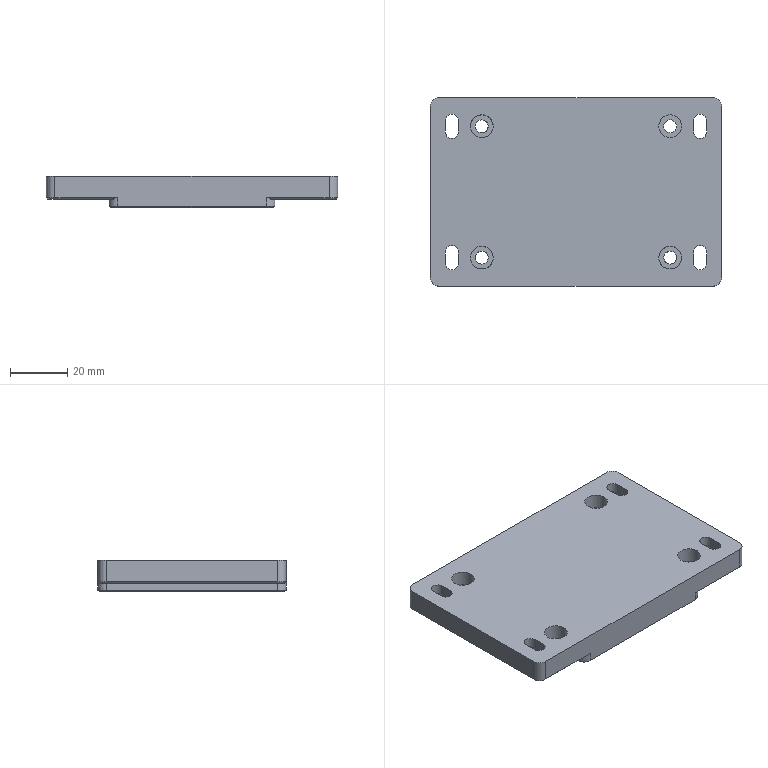Part | 1 solid | 84 faces | box 102 x 66 x 11 mm | volume 62010 mm3 | plane 44 | cylinder 32 | cone 8 | commonest cylinder face diameters 4.5 x12 8 x12 6 x8